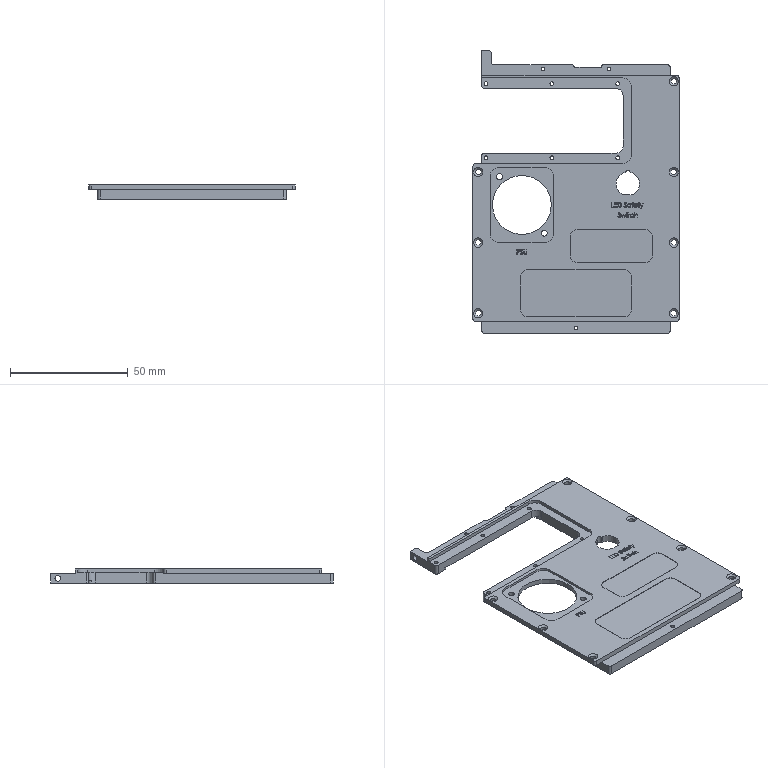NC program | NX | posted with a generic post | part box 87.5 x 120 x 6.001 mm
Lines 4765 to 5363 of 10039:
(CAVITY_MILL_1 , TOOL : D3-12-D3-75-3T)
N9492 T20 M6
N9494 G53
N9496 G17 G0 G90 X50.4 Y-32.135 B0. C0. S6500 M3
N9498 G43 Z5. H20
N9500 Z-0.7
N9502 G94 G1 Y-36.4 Z-0.849 F2600.
N9504 X49.576 Z-0.878
N9506 X49.523 Y-36.008 Z-0.892
N9508 X49.2 Y-35.309 Z-0.918
N9510 X48.688 Y-34.733 Z-0.945
N9512 X48.284 Y-34.489 Z-0.962
N9514 X47.961 Y-34.306 Z-0.975
N9516 X47.6 Y-34.22 Z-0.988
N9518 Y-26.096 Z-1.271
N9520 Y-14.28
N9522 G3 X48.4 Y-13.941 R2.6
N9524 G1 Y-15.5
N9526 G3 X50.4 Y-18.03 R2.6
N9528 G1 Y-34.914
N9530 Y-35.
N9532 Y-36.4
N9534 X49.576
N9536 G3 X47.6 Y-34.22 R2.6
N9538 G1 Y-26.096
N9540 X48.95
N9542 Y-18.876
N9544 X49.05 Y-18.935
N9546 Y-33.374
N9548 X48.95 Y-33.315
N9550 Y-26.096
N9552 Z-0.971
N9554 G0 X50.4 Y-32.135
N9556 G1 Y-36.4 Z-1.12
N9558 X49.576 Z-1.149
N9560 X49.523 Y-36.008 Z-1.163
N9562 X49.2 Y-35.309 Z-1.19
N9564 X48.688 Y-34.733 Z-1.217
N9566 X48.284 Y-34.489 Z-1.233
N9568 X47.961 Y-34.306 Z-1.246
N9570 X47.6 Y-34.22 Z-1.259
N9572 Y-26.096 Z-1.543
N9574 Y-14.28
N9576 G3 X48.4 Y-13.941 R2.6
N9578 G1 Y-15.5
N9580 G3 X50.4 Y-18.03 R2.6
N9582 G1 Y-36.4
N9584 X49.576
N9586 G3 X47.6 Y-34.22 R2.6
N9588 G1 Y-26.096
N9590 X48.95
N9592 Y-18.876
N9594 X49.05 Y-18.935
N9596 Y-33.374
N9598 X48.95 Y-33.315
N9600 Y-26.096
N9602 Z-1.243
N9604 G0 X50.4 Y-32.135
N9606 G1 Y-36.4 Z-1.392
N9608 X49.576 Z-1.421
N9610 X49.523 Y-36.008 Z-1.434
N9612 X49.2 Y-35.309 Z-1.461
N9614 X48.688 Y-34.733 Z-1.488
N9616 X48.284 Y-34.489 Z-1.505
N9618 X47.961 Y-34.306 Z-1.518
N9620 X47.6 Y-34.22 Z-1.531
N9622 Y-26.096 Z-1.814
N9624 Y-14.28
N9626 G3 X48.4 Y-13.941 R2.6
N9628 G1 Y-15.5
N9630 G3 X50.4 Y-18.03 R2.6
N9632 G1 Y-36.4
N9634 X49.576
N9636 G3 X47.6 Y-34.22 R2.6
N9638 G1 Y-26.096
N9640 X48.95
N9642 Y-18.876
N9644 X49.05 Y-18.935
N9646 Y-33.374
N9648 X48.95 Y-33.315
N9650 Y-26.096
N9652 Z-1.514
N9654 G0 X50.4 Y-32.135
N9656 G1 Y-36.4 Z-1.663
N9658 X49.576 Z-1.692
N9660 X49.523 Y-36.008 Z-1.706
N9662 X49.2 Y-35.309 Z-1.733
N9664 X48.688 Y-34.733 Z-1.76
N9666 X48.284 Y-34.489 Z-1.776
N9668 X47.961 Y-34.306 Z-1.789
N9670 X47.6 Y-34.22 Z-1.802
N9672 Y-26.096 Z-2.086
N9674 Y-14.28
N9676 G3 X48.4 Y-13.941 R2.6
N9678 G1 Y-15.5
N9680 G3 X50.4 Y-18.03 R2.6
N9682 G1 Y-36.4
N9684 X49.576
N9686 G3 X47.6 Y-34.22 R2.6
N9688 G1 Y-26.096
N9690 X48.95
N9692 Y-18.876
N9694 X49.05 Y-18.935
N9696 Y-33.374
N9698 X48.95 Y-33.315
N9700 Y-26.096
N9702 Z-1.786
N9704 G0 X50.4 Y-32.135
N9706 G1 Y-36.4 Z-1.935
N9708 X49.576 Z-1.963
N9710 X49.523 Y-36.008 Z-1.977
N9712 X49.2 Y-35.309 Z-2.004
N9714 X48.688 Y-34.733 Z-2.031
N9716 X48.284 Y-34.489 Z-2.048
N9718 X47.961 Y-34.306 Z-2.06
N9720 X47.6 Y-34.22 Z-2.073
N9722 Y-26.096 Z-2.357
N9724 Y-14.28
N9726 G3 X48.4 Y-13.941 R2.6
N9728 G1 Y-15.5
N9730 G3 X50.4 Y-18.03 R2.6
N9732 G1 Y-36.4
N9734 X49.576
N9736 G3 X47.6 Y-34.22 R2.6
N9738 G1 Y-26.096
N9740 X48.95
N9742 Y-18.876
N9744 X49.05 Y-18.935
N9746 Y-33.374
N9748 X48.95 Y-33.315
N9750 Y-26.096
N9752 Z-2.057
N9754 G0 X50.4 Y-32.135
N9756 G1 Y-36.4 Z-2.206
N9758 X49.576 Z-2.235
N9760 X49.523 Y-36.008 Z-2.249
N9762 X49.2 Y-35.309 Z-2.276
N9764 X48.688 Y-34.733 Z-2.302
N9766 X48.284 Y-34.489 Z-2.319
N9768 X47.961 Y-34.306 Z-2.332
N9770 X47.6 Y-34.22 Z-2.345
N9772 Y-26.096 Z-2.629
N9774 Y-14.28
N9776 G3 X48.4 Y-13.941 R2.6
N9778 G1 Y-15.5
N9780 G3 X50.4 Y-18.03 R2.6
N9782 G1 Y-36.4
N9784 X49.576
N9786 G3 X47.6 Y-34.22 R2.6
N9788 G1 Y-26.096
N9790 X48.95
N9792 Y-18.876
N9794 X49.05 Y-18.935
N9796 Y-33.374
N9798 X48.95 Y-33.315
N9800 Y-26.096
N9802 Z-2.329
N9804 G0 X50.4 Y-32.135
N9806 G1 Y-36.4 Z-2.477
N9808 X49.576 Z-2.506
N9810 X49.523 Y-36.008 Z-2.52
N9812 X49.2 Y-35.309 Z-2.547
N9814 X48.688 Y-34.733 Z-2.574
N9816 X48.284 Y-34.489 Z-2.59
N9818 X47.961 Y-34.306 Z-2.603
N9820 X47.6 Y-34.22 Z-2.616
N9822 Y-26.096 Z-2.9
N9824 Y-14.28
N9826 G3 X48.4 Y-13.941 R2.6
N9828 G1 Y-15.5
N9830 G3 X50.4 Y-18.03 R2.6
N9832 G1 Y-36.4
N9834 X49.576
N9836 G3 X47.6 Y-34.22 R2.6
N9838 G1 Y-26.096
N9840 X48.95
N9842 Y-18.876
N9844 X49.05 Y-18.935
N9846 Y-33.374
N9848 X48.95 Y-33.315
N9850 Y-26.096
N9852 Z-2.6
N9854 G0 Z5.
N9856 X47.6 Y10.513
N9858 Z-0.7
N9860 G1 Y13.72 Z-0.812
N9862 X47.985 Y13.812 Z-0.826
N9864 X48.066 Y13.846 Z-0.829
N9866 X48.4 Y14.059 Z-0.843
N9868 Y12.5 Z-0.897
N9870 Y12.104 Z-0.911
N9872 X48.668 Y11.284 Z-0.941
N9874 X49.187 Y10.595 Z-0.971
N9876 X49.9 Y10.111 Z-1.001
N9878 X50.508 Y9.936 Z-1.023
N9880 X50.743 Y9.913 Z-1.032
N9882 X51.012 Y9.679 Z-1.044
N9884 X51.17 Y9.593 Z-1.05
N9886 X51.808 Y9.4 Z-1.074
N9888 X53.003 Z-1.115
N9890 Y4.932 Z-1.271
N9892 Y0.6
N9894 X52.5
N9896 G3 X50.4 Y-1.5 R2.1
N9898 G1 Y-9.97
N9900 G3 X49.6 Y-10.309 R2.6
N9902 G1 Y-8.75
N9904 G3 X47.6 Y-6.22 R2.6
N9906 G1 Y13.72
N9908 G3 X48.4 Y14.059 R2.6
N9910 G1 Y12.5
N9912 G3 X50.743 Y9.913 R2.6
N9914 X52.118 Y9.4 R2.1
N9916 G1 X53.003
N9918 Y4.932
N9920 X50.903
N9922 Y2.385
N9924 G3 X49.7 Y1.63 R4.2
N9926 G1 X49.17 Y0.045
N9928 X49.7 Y1.63
N9930 Y7.983
N9932 G3 X49.908 Y7.929 R4.7
N9934 X50.903 Y7.48 R4.2
N9936 G1 Y4.932
N9938 Z-0.971
N9940 G0 X47.6 Y10.513
N9942 G1 Y13.72 Z-1.083
N9944 X47.985 Y13.812 Z-1.097
N9946 X48.066 Y13.846 Z-1.1
N9948 X48.4 Y14.059 Z-1.114
N9950 Y12.104 Z-1.182
N9952 X48.668 Y11.284 Z-1.213
N9954 X49.187 Y10.595 Z-1.243
N9956 X49.9 Y10.111 Z-1.273
N9958 X50.508 Y9.936 Z-1.295
N9960 X50.743 Y9.913 Z-1.303
N9962 X51.012 Y9.679 Z-1.316
N9964 X51.17 Y9.593 Z-1.322
N9966 X51.808 Y9.4 Z-1.345
N9968 X53.003 Z-1.387
N9970 Y4.932 Z-1.543
N9972 Y0.6
N9974 X52.5
N9976 G3 X50.4 Y-1.5 R2.1
N9978 G1 Y-9.97
N9980 G3 X49.6 Y-10.309 R2.6
N9982 G1 Y-8.75
N9984 G3 X47.6 Y-6.22 R2.6
N9986 G1 Y13.72
N9988 G3 X48.4 Y14.059 R2.6
N9990 G1 Y12.5
N9992 G3 X50.743 Y9.913 R2.6
N9994 X52.118 Y9.4 R2.1
N9996 G1 X53.003
N9998 Y4.932
N10000 X50.903
N10002 Y2.385
N10004 G3 X49.7 Y1.63 R4.2
N10006 G1 X49.17 Y0.045
N10008 X49.7 Y1.63
N10010 Y7.983
N10012 G3 X49.908 Y7.929 R4.7
N10014 X50.903 Y7.48 R4.2
N10016 G1 Y4.932
N10018 Z-1.243
N10020 G0 X47.6 Y10.513
N10022 G1 Y13.72 Z-1.355
N10024 X47.985 Y13.812 Z-1.369
N10026 X48.066 Y13.846 Z-1.372
N10028 X48.4 Y14.059 Z-1.386
N10030 Y12.5 Z-1.44
N10032 Y12.104 Z-1.454
N10034 X48.668 Y11.284 Z-1.484
N10036 X49.187 Y10.595 Z-1.514
N10038 X49.9 Y10.111 Z-1.544
N10040 X50.508 Y9.936 Z-1.566
N10042 X50.743 Y9.913 Z-1.575
N10044 X51.012 Y9.679 Z-1.587
N10046 X51.17 Y9.593 Z-1.593
N10048 X51.808 Y9.4 Z-1.617
N10050 X53.003 Z-1.658
N10052 Y4.932 Z-1.814
N10054 Y0.6
N10056 X52.5
N10058 G3 X50.4 Y-1.5 R2.1
N10060 G1 Y-9.97
N10062 G3 X49.6 Y-10.309 R2.6
N10064 G1 Y-8.75
N10066 G3 X47.6 Y-6.22 R2.6
N10068 G1 Y13.72
N10070 G3 X48.4 Y14.059 R2.6
N10072 G1 Y12.5
N10074 G3 X50.743 Y9.913 R2.6
N10076 X52.118 Y9.4 R2.1
N10078 G1 X53.003
N10080 Y4.932
N10082 X50.903
N10084 Y2.385
N10086 G3 X49.7 Y1.63 R4.2
N10088 G1 X49.17 Y0.045
N10090 X49.7 Y1.63
N10092 Y7.983
N10094 G3 X49.908 Y7.929 R4.7
N10096 X50.903 Y7.48 R4.2
N10098 G1 Y4.932
N10100 Z-1.514
N10102 G0 X47.6 Y10.513
N10104 G1 Y13.72 Z-1.626
N10106 X47.985 Y13.812 Z-1.64
N10108 X48.066 Y13.846 Z-1.643
N10110 X48.4 Y14.059 Z-1.657
N10112 Y12.104 Z-1.725
N10114 X48.668 Y11.284 Z-1.755
N10116 X49.187 Y10.595 Z-1.786
N10118 X49.9 Y10.111 Z-1.816
N10120 X50.508 Y9.936 Z-1.838
N10122 X50.743 Y9.913 Z-1.846
N10124 X51.012 Y9.679 Z-1.858
N10126 X51.17 Y9.593 Z-1.865
N10128 X51.808 Y9.4 Z-1.888
N10130 X53.003 Z-1.93
N10132 Y4.932 Z-2.086
N10134 Y0.6
N10136 X52.5
N10138 G3 X50.4 Y-1.5 R2.1
N10140 G1 Y-9.97
N10142 G3 X49.6 Y-10.309 R2.6
N10144 G1 Y-8.75
N10146 G3 X47.6 Y-6.22 R2.6
N10148 G1 Y13.72
N10150 G3 X48.4 Y14.059 R2.6
N10152 G1 Y12.5
N10154 G3 X50.743 Y9.913 R2.6
N10156 X52.118 Y9.4 R2.1
N10158 G1 X53.003
N10160 Y4.932
N10162 X50.903
N10164 Y2.385
N10166 G3 X49.7 Y1.63 R4.2
N10168 G1 X49.17 Y0.045
N10170 X49.7 Y1.63
N10172 Y7.983
N10174 G3 X49.908 Y7.929 R4.7
N10176 X50.903 Y7.48 R4.2
N10178 G1 Y4.932
N10180 Z-1.786
N10182 G0 X47.6 Y10.513
N10184 G1 Y13.72 Z-1.898
N10186 X47.985 Y13.812 Z-1.912
N10188 X48.066 Y13.846 Z-1.915
N10190 X48.4 Y14.059 Z-1.928
N10192 Y12.104 Z-1.997
N10194 X48.668 Y11.284 Z-2.027
N10196 X49.187 Y10.595 Z-2.057
N10198 X49.9 Y10.111 Z-2.087
N10200 X50.508 Y9.936 Z-2.109
N10202 X50.743 Y9.913 Z-2.117
N10204 X51.012 Y9.679 Z-2.13
N10206 X51.17 Y9.593 Z-2.136
N10208 X51.808 Y9.4 Z-2.159
N10210 X53.003 Z-2.201
N10212 Y4.932 Z-2.357
N10214 Y0.6
N10216 X52.5
N10218 G3 X50.4 Y-1.5 R2.1
N10220 G1 Y-9.97
N10222 G3 X49.6 Y-10.309 R2.6
N10224 G1 Y-8.75
N10226 G3 X47.6 Y-6.22 R2.6
N10228 G1 Y13.72
N10230 G3 X48.4 Y14.059 R2.6
N10232 G1 Y12.5
N10234 G3 X50.743 Y9.913 R2.6
N10236 X52.118 Y9.4 R2.1
N10238 G1 X53.003
N10240 Y4.932
N10242 X50.903
N10244 Y2.385
N10246 G3 X49.7 Y1.63 R4.2
N10248 G1 X49.17 Y0.045
N10250 X49.7 Y1.63
N10252 Y7.983
N10254 G3 X49.908 Y7.929 R4.7
N10256 X50.903 Y7.48 R4.2
N10258 G1 Y4.932
N10260 Z-2.057
N10262 G0 X47.6 Y10.513
N10264 G1 Y13.72 Z-2.169
N10266 X47.985 Y13.812 Z-2.183
N10268 X48.066 Y13.846 Z-2.186
N10270 X48.4 Y14.059 Z-2.2
N10272 Y12.104 Z-2.268
N10274 X48.668 Y11.284 Z-2.298
N10276 X49.187 Y10.595 Z-2.328
N10278 X49.9 Y10.111 Z-2.358
N10280 X50.508 Y9.936 Z-2.381
N10282 X50.743 Y9.913 Z-2.389
N10284 X51.012 Y9.679 Z-2.401
N10286 X51.17 Y9.593 Z-2.408
N10288 X51.808 Y9.4 Z-2.431
N10290 X53.003 Z-2.473
N10292 Y4.932 Z-2.629
N10294 Y0.6
N10296 X52.5
N10298 G3 X50.4 Y-1.5 R2.1
N10300 G1 Y-9.97
N10302 G3 X49.6 Y-10.309 R2.6
N10304 G1 Y-8.75
N10306 G3 X47.6 Y-6.22 R2.6
N10308 G1 Y13.72
N10310 G3 X48.4 Y14.059 R2.6
N10312 G1 Y12.5
N10314 G3 X50.743 Y9.913 R2.6
N10316 X52.118 Y9.4 R2.1
N10318 G1 X53.003
N10320 Y4.932
N10322 X50.903
N10324 Y2.385
N10326 G3 X49.7 Y1.63 R4.2
N10328 G1 X49.17 Y0.045
N10330 X49.7 Y1.63
N10332 Y7.983
N10334 G3 X49.908 Y7.929 R4.7
N10336 X50.903 Y7.48 R4.2
N10338 G1 Y4.932
N10340 Z-2.329
N10342 G0 X47.6 Y10.513
N10344 G1 Y13.72 Z-2.441
N10346 X47.985 Y13.812 Z-2.454
N10348 X48.066 Y13.846 Z-2.457
N10350 X48.4 Y14.059 Z-2.471
N10352 Y12.5 Z-2.526
N10354 Y12.104 Z-2.54
N10356 X48.668 Y11.284 Z-2.57
N10358 X49.187 Y10.595 Z-2.6
N10360 X49.9 Y10.111 Z-2.63
N10362 X50.508 Y9.936 Z-2.652
N10364 X50.743 Y9.913 Z-2.66
N10366 X51.012 Y9.679 Z-2.673
N10368 X51.17 Y9.593 Z-2.679
N10370 X51.808 Y9.4 Z-2.702
N10372 X53.003 Z-2.744
N10374 Y4.932 Z-2.9
N10376 Y0.6
N10378 X52.5
N10380 G3 X50.4 Y-1.5 R2.1
N10382 G1 Y-9.97
N10384 G3 X49.6 Y-10.309 R2.6
N10386 G1 Y-8.75
N10388 G3 X47.6 Y-6.22 R2.6
N10390 G1 Y13.72
N10392 G3 X48.4 Y14.059 R2.6
N10394 G1 Y12.5
N10396 G3 X50.743 Y9.913 R2.6
N10398 X52.118 Y9.4 R2.1
N10400 G1 X53.003
N10402 Y4.932
N10404 X50.903
N10406 Y2.385
N10408 G3 X49.7 Y1.63 R4.2
N10410 G1 X49.17 Y0.045
N10412 X49.7 Y1.63
N10414 Y7.983
N10416 G3 X49.908 Y7.929 R4.7
N10418 X50.903 Y7.48 R4.2
N10420 G1 Y4.932
N10422 Z-2.6
N10424 G0 Z5.
N10426 X47.6 Y30.398
N10428 Z-0.7
N10430 G1 Y36.4 Z-0.91
N10432 X50.4 Z-1.007
N10434 Y28.838 Z-1.271
N10436 Y18.03
N10438 G3 X49.6 Y17.691 R2.6
N10440 G1 Y19.25
N10442 G3 X47.6 Y21.78 R2.6
N10444 G1 Y36.4
N10446 X50.4
N10448 Y28.838
N10450 X49.05
N10452 Y22.626
N10454 X48.95 Y22.685
N10456 Y35.05
N10458 X49.05
N10460 Y28.838
N10462 Z-0.971
N10464 G0 X47.6 Y30.398
N10466 G1 Y36.4 Z-1.181
N10468 X50.4 Z-1.279
N10470 Y28.838 Z-1.543
N10472 Y18.03
N10474 G3 X49.6 Y17.691 R2.6
N10476 G1 Y19.25
N10478 G3 X47.6 Y21.78 R2.6
N10480 G1 Y36.4
N10482 X50.4
N10484 Y28.838
N10486 X49.05
N10488 Y22.626
N10490 X48.95 Y22.685
N10492 Y35.05
N10494 X49.05
N10496 Y28.838
N10498 Z-1.243
N10500 G0 X47.6 Y30.398
N10502 G1 Y36.4 Z-1.452
N10504 X50.4 Z-1.55
N10506 Y28.838 Z-1.814
N10508 Y18.03
N10510 G3 X49.6 Y17.691 R2.6
N10512 G1 Y19.25
N10514 G3 X47.6 Y21.78 R2.6
N10516 G1 Y36.4
N10518 X50.4
N10520 Y28.838
N10522 X49.05
N10524 Y22.626
N10526 X48.95 Y22.685
N10528 Y35.05
N10530 X49.05
N10532 Y28.838
N10534 Z-1.514
N10536 G0 X47.6 Y30.398
N10538 G1 Y36.4 Z-1.724
N10540 X50.4 Z-1.822
N10542 Y28.838 Z-2.086
N10544 Y18.03
N10546 G3 X49.6 Y17.691 R2.6
N10548 G1 Y19.25
N10550 G3 X47.6 Y21.78 R2.6
N10552 G1 Y36.4
N10554 X50.4
N10556 Y28.838
N10558 X49.05
N10560 Y22.626
N10562 X48.95 Y22.685
N10564 Y35.05
N10566 X49.05
N10568 Y28.838
N10570 Z-1.786
N10572 G0 X47.6 Y30.398
N10574 G1 Y36.4 Z-1.995
N10576 X50.4 Z-2.093
N10578 Y28.838 Z-2.357
N10580 Y18.03
N10582 G3 X49.6 Y17.691 R2.6
N10584 G1 Y19.25
N10586 G3 X47.6 Y21.78 R2.6
N10588 G1 Y36.4
N10590 X50.4
N10592 Y28.838
N10594 X49.05
N10596 Y22.626
N10598 X48.95 Y22.685
N10600 Y35.05
N10602 X49.05
N10604 Y28.838
N10606 Z-2.057
N10608 G0 X47.6 Y30.398
N10610 G1 Y36.4 Z-2.267
N10612 X50.4 Z-2.365
N10614 Y28.838 Z-2.629
N10616 Y18.03
N10618 G3 X49.6 Y17.691 R2.6
N10620 G1 Y19.25
N10622 G3 X47.6 Y21.78 R2.6
N10624 G1 Y36.4
N10626 X50.4
N10628 Y28.838
N10630 X49.05
N10632 Y22.626
N10634 X48.95 Y22.685
N10636 Y35.05
N10638 X49.05
N10640 Y28.838
N10642 Z-2.329
N10644 G0 X47.6 Y30.398
N10646 G1 Y36.4 Z-2.538
N10648 X50.4 Z-2.636
N10650 Y28.838 Z-2.9
N10652 Y18.03
N10654 G3 X49.6 Y17.691 R2.6
N10656 G1 Y19.25
N10658 G3 X47.6 Y21.78 R2.6
N10660 G1 Y36.4
N10662 X50.4
N10664 Y28.838
N10666 X49.05
N10668 Y22.626
N10670 X48.95 Y22.685
N10672 Y35.05
N10674 X49.05
N10676 Y28.838
N10678 Z-2.6
N10680 G0 Z5.
N10682 M5